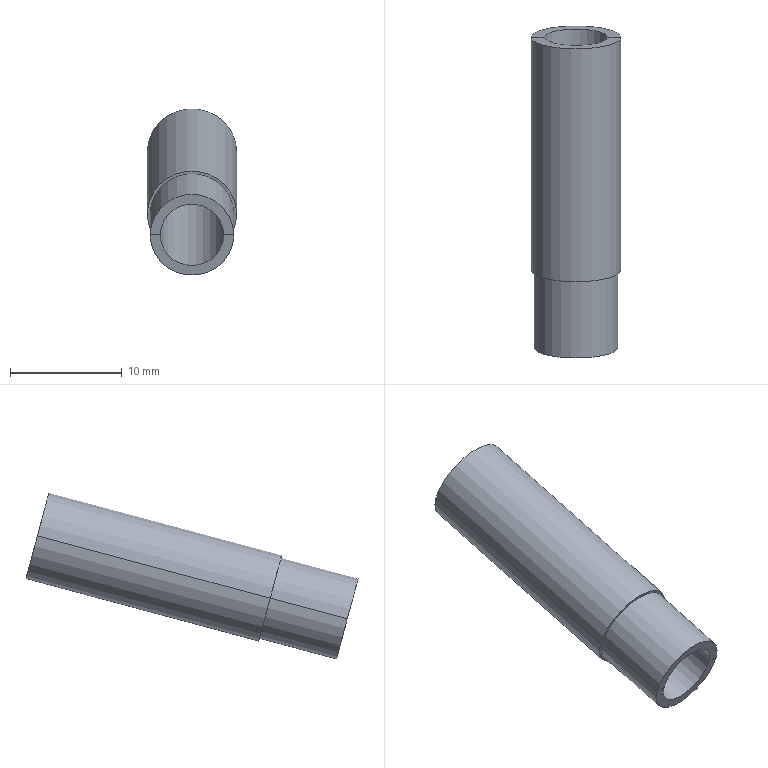Part | STEP file | BREP_2 | 1 solid | 12 faces | box 8 x 29.756 x 14.922 mm | volume 672.27 mm3 | cylinder 6 | plane 6 | commonest cylinder face diameters 5.681 x2 7.5 x2 8 x2
STEP:
#1=CARTESIAN_POINT('',(0.,0.,0.));
#2=DIRECTION('',(0.,0.,1.));
#3=DIRECTION('',(1.,0.,0.));
#4=AXIS2_PLACEMENT_3D('',#1,#2,#3);
#5=CARTESIAN_POINT('',(2.841,186.663,50.016));
#6=VERTEX_POINT('',#5);
#7=CARTESIAN_POINT('',(-2.841,186.663,50.016));
#8=VERTEX_POINT('',#7);
#9=CARTESIAN_POINT('',(0.,186.663,50.016));
#10=DIRECTION('',(0.,0.9659,0.2588));
#11=DIRECTION('',(1.,0.,0.));
#12=AXIS2_PLACEMENT_3D('',#9,#10,#11);
#13=CIRCLE('',#12,2.841);
#14=CARTESIAN_POINT('',(0.,200.538,53.734));
#15=DIRECTION('',(0.,0.9659,0.2588));
#16=DIRECTION('',(1.,0.,0.));
#17=AXIS2_PLACEMENT_3D('',#14,#15,#16);
#18=CYLINDRICAL_SURFACE('',#17,2.841);
#19=CARTESIAN_POINT('',(0.,-14.365));
#20=DIRECTION('',(1.,0.));
#21=VECTOR('',#20,1.);
#22=LINE('',#19,#21);
#23=(GEOMETRIC_REPRESENTATION_CONTEXT(2)PARAMETRIC_REPRESENTATION_CONTEXT()REPRESENTATION_CONTEXT('',''));
#24=DEFINITIONAL_REPRESENTATION('',(#22),#23);
#25=PCURVE('',#18,#24);
#26=CARTESIAN_POINT('',(0.,187.516,46.833));
#27=DIRECTION('',(0.,0.9659,0.2588));
#28=DIRECTION('',(0.,-0.2588,0.9659));
#29=AXIS2_PLACEMENT_3D('',#26,#27,#28);
#30=PLANE('',#29);
#31=CARTESIAN_POINT('',(3.295,0.));
#32=DIRECTION('',(0.,1.));
#33=AXIS2_PLACEMENT_2D('',#31,#32);
#34=CIRCLE('',#33,2.841);
#35=(GEOMETRIC_REPRESENTATION_CONTEXT(2)PARAMETRIC_REPRESENTATION_CONTEXT()REPRESENTATION_CONTEXT('',''));
#36=DEFINITIONAL_REPRESENTATION('',(#34),#35);
#37=PCURVE('',#30,#36);
#38=SURFACE_CURVE('',#13,(#25,#37),.PCURVE_S1.);
#39=EDGE_CURVE('',#6,#8,#38,.T.);
#40=ORIENTED_EDGE('',*,*,#39,.T.);
#41=CARTESIAN_POINT('',(-2.841,214.414,57.452));
#42=VERTEX_POINT('',#41);
#43=CARTESIAN_POINT('',(-2.841,214.414,57.452));
#44=DIRECTION('',(0.,-0.9659,-0.2588));
#45=VECTOR('',#44,1.);
#46=LINE('',#43,#45);
#47=CARTESIAN_POINT('',(3.142,14.365));
#48=DIRECTION('',(0.,-1.));
#49=VECTOR('',#48,1.);
#50=LINE('',#47,#49);
#51=(GEOMETRIC_REPRESENTATION_CONTEXT(2)PARAMETRIC_REPRESENTATION_CONTEXT()REPRESENTATION_CONTEXT('',''));
#52=DEFINITIONAL_REPRESENTATION('',(#50),#51);
#53=PCURVE('',#18,#52);
#54=CARTESIAN_POINT('',(0.,200.538,53.734));
#55=DIRECTION('',(0.,0.9659,0.2588));
#56=DIRECTION('',(-1.,0.,0.));
#57=AXIS2_PLACEMENT_3D('',#54,#55,#56);
#58=CYLINDRICAL_SURFACE('',#57,2.841);
#59=CARTESIAN_POINT('',(0.,14.365));
#60=DIRECTION('',(0.,-1.));
#61=VECTOR('',#60,1.);
#62=LINE('',#59,#61);
#63=(GEOMETRIC_REPRESENTATION_CONTEXT(2)PARAMETRIC_REPRESENTATION_CONTEXT()REPRESENTATION_CONTEXT('',''));
#64=DEFINITIONAL_REPRESENTATION('',(#62),#63);
#65=PCURVE('',#58,#64);
#66=SURFACE_CURVE('',#46,(#53,#65),.PCURVE_S1.);
#67=EDGE_CURVE('',#42,#8,#66,.T.);
#68=ORIENTED_EDGE('',*,*,#67,.F.);
#69=CARTESIAN_POINT('',(2.841,214.414,57.452));
#70=VERTEX_POINT('',#69);
#71=CARTESIAN_POINT('',(0.,214.414,57.452));
#72=DIRECTION('',(0.,-0.9659,-0.2588));
#73=DIRECTION('',(-1.,0.,0.));
#74=AXIS2_PLACEMENT_3D('',#71,#72,#73);
#75=CIRCLE('',#74,2.841);
#76=CARTESIAN_POINT('',(3.142,14.365));
#77=DIRECTION('',(-1.,0.));
#78=VECTOR('',#77,1.);
#79=LINE('',#76,#78);
#80=(GEOMETRIC_REPRESENTATION_CONTEXT(2)PARAMETRIC_REPRESENTATION_CONTEXT()REPRESENTATION_CONTEXT('',''));
#81=DEFINITIONAL_REPRESENTATION('',(#79),#80);
#82=PCURVE('',#18,#81);
#83=CARTESIAN_POINT('',(0.,215.299,54.148));
#84=DIRECTION('',(0.,0.9659,0.2588));
#85=DIRECTION('',(0.,0.2588,-0.9659));
#86=AXIS2_PLACEMENT_3D('',#83,#84,#85);
#87=PLANE('',#86);
#88=CARTESIAN_POINT('',(-3.42,2.841));
#89=CARTESIAN_POINT('',(1.5,2.841));
#90=CARTESIAN_POINT('',(-0.9602,-1.42));
#91=CARTESIAN_POINT('',(-3.42,-5.681));
#92=CARTESIAN_POINT('',(-5.88,-1.42));
#93=CARTESIAN_POINT('',(-8.341,2.841));
#94=CARTESIAN_POINT('',(-3.42,2.841));
#95=(BOUNDED_CURVE()B_SPLINE_CURVE(2,(#88,#89,#90,#91,#92,#93,#94),.UNSPECIFIED.,.T.,.F.)B_SPLINE_CURVE_WITH_KNOTS((1,2,2,2,2,1),(-2.094,0.,2.094,4.189,6.283,8.378),.UNSPECIFIED.)CURVE()GEOMETRIC_REPRESENTATION_ITEM()RATIONAL_B_SPLINE_CURVE((1.,0.5,1.,0.5,1.,0.5,1.))REPRESENTATION_ITEM(''));
#96=(GEOMETRIC_REPRESENTATION_CONTEXT(2)PARAMETRIC_REPRESENTATION_CONTEXT()REPRESENTATION_CONTEXT('',''));
#97=DEFINITIONAL_REPRESENTATION('',(#95),#96);
#98=PCURVE('',#87,#97);
#99=SURFACE_CURVE('',#75,(#82,#98),.PCURVE_S1.);
#100=EDGE_CURVE('',#42,#70,#99,.T.);
#101=ORIENTED_EDGE('',*,*,#100,.T.);
#102=CARTESIAN_POINT('',(2.841,214.414,57.452));
#103=DIRECTION('',(0.,-0.9659,-0.2588));
#104=VECTOR('',#103,1.);
#105=LINE('',#102,#104);
#106=CARTESIAN_POINT('',(0.,14.365));
#107=DIRECTION('',(0.,-1.));
#108=VECTOR('',#107,1.);
#109=LINE('',#106,#108);
#110=(GEOMETRIC_REPRESENTATION_CONTEXT(2)PARAMETRIC_REPRESENTATION_CONTEXT()REPRESENTATION_CONTEXT('',''));
#111=DEFINITIONAL_REPRESENTATION('',(#109),#110);
#112=PCURVE('',#18,#111);
#113=CARTESIAN_POINT('',(3.142,14.365));
#114=DIRECTION('',(0.,-1.));
#115=VECTOR('',#114,1.);
#116=LINE('',#113,#115);
#117=(GEOMETRIC_REPRESENTATION_CONTEXT(2)PARAMETRIC_REPRESENTATION_CONTEXT()REPRESENTATION_CONTEXT('',''));
#118=DEFINITIONAL_REPRESENTATION('',(#116),#117);
#119=PCURVE('',#58,#118);
#120=SURFACE_CURVE('',#105,(#112,#119),.PCURVE_S1.);
#121=EDGE_CURVE('',#70,#6,#120,.T.);
#122=ORIENTED_EDGE('',*,*,#121,.T.);
#123=EDGE_LOOP('',(#40,#68,#101,#122));
#124=FACE_BOUND('',#123,.F.);
#125=ADVANCED_FACE('',(#124),#18,.F.);
#126=CARTESIAN_POINT('',(-3.75,186.663,50.016));
#127=VERTEX_POINT('',#126);
#128=CARTESIAN_POINT('',(3.75,186.663,50.016));
#129=VERTEX_POINT('',#128);
#130=CARTESIAN_POINT('',(0.,186.663,50.016));
#131=DIRECTION('',(0.,-0.9659,-0.2588));
#132=DIRECTION('',(-1.,0.,0.));
#133=AXIS2_PLACEMENT_3D('',#130,#131,#132);
#134=CIRCLE('',#133,3.75);
#135=CARTESIAN_POINT('',(3.295,-3.75));
#136=CARTESIAN_POINT('',(-3.2,-3.75));
#137=CARTESIAN_POINT('',(0.04775,1.875));
#138=CARTESIAN_POINT('',(3.295,7.5));
#139=CARTESIAN_POINT('',(6.543,1.875));
#140=CARTESIAN_POINT('',(9.791,-3.75));
#141=CARTESIAN_POINT('',(3.295,-3.75));
#142=(BOUNDED_CURVE()B_SPLINE_CURVE(2,(#135,#136,#137,#138,#139,#140,#141),.UNSPECIFIED.,.T.,.F.)B_SPLINE_CURVE_WITH_KNOTS((1,2,2,2,2,1),(-2.094,0.,2.094,4.189,6.283,8.378),.UNSPECIFIED.)CURVE()GEOMETRIC_REPRESENTATION_ITEM()RATIONAL_B_SPLINE_CURVE((1.,0.5,1.,0.5,1.,0.5,1.))REPRESENTATION_ITEM(''));
#143=(GEOMETRIC_REPRESENTATION_CONTEXT(2)PARAMETRIC_REPRESENTATION_CONTEXT()REPRESENTATION_CONTEXT('',''));
#144=DEFINITIONAL_REPRESENTATION('',(#142),#143);
#145=PCURVE('',#30,#144);
#146=CARTESIAN_POINT('',(0.,190.115,50.941));
#147=DIRECTION('',(0.,-0.9659,-0.2588));
#148=DIRECTION('',(1.,0.,0.));
#149=AXIS2_PLACEMENT_3D('',#146,#147,#148);
#150=CYLINDRICAL_SURFACE('',#149,3.75);
#151=CARTESIAN_POINT('',(3.142,3.573));
#152=DIRECTION('',(1.,0.));
#153=VECTOR('',#152,1.);
#154=LINE('',#151,#153);
#155=(GEOMETRIC_REPRESENTATION_CONTEXT(2)PARAMETRIC_REPRESENTATION_CONTEXT()REPRESENTATION_CONTEXT('',''));
#156=DEFINITIONAL_REPRESENTATION('',(#154),#155);
#157=PCURVE('',#150,#156);
#158=SURFACE_CURVE('',#134,(#145,#157),.PCURVE_S1.);
#159=EDGE_CURVE('',#127,#129,#158,.T.);
#160=ORIENTED_EDGE('',*,*,#159,.F.);
#161=CARTESIAN_POINT('',(-2.841,186.663,50.016));
#162=DIRECTION('',(-1.,0.,0.));
#163=VECTOR('',#162,1.);
#164=LINE('',#161,#163);
#165=CARTESIAN_POINT('',(3.295,-2.841));
#166=DIRECTION('',(0.,-1.));
#167=VECTOR('',#166,1.);
#168=LINE('',#165,#167);
#169=(GEOMETRIC_REPRESENTATION_CONTEXT(2)PARAMETRIC_REPRESENTATION_CONTEXT()REPRESENTATION_CONTEXT('',''));
#170=DEFINITIONAL_REPRESENTATION('',(#168),#169);
#171=PCURVE('',#30,#170);
#172=CARTESIAN_POINT('',(0.,185.81,53.199));
#173=DIRECTION('',(0.,0.9659,0.2588));
#174=DIRECTION('',(0.,0.2588,-0.9659));
#175=AXIS2_PLACEMENT_3D('',#172,#173,#174);
#176=PLANE('',#175);
#177=CARTESIAN_POINT('',(3.295,2.841));
#178=DIRECTION('',(0.,1.));
#179=VECTOR('',#178,1.);
#180=LINE('',#177,#179);
#181=(GEOMETRIC_REPRESENTATION_CONTEXT(2)PARAMETRIC_REPRESENTATION_CONTEXT()REPRESENTATION_CONTEXT('',''));
#182=DEFINITIONAL_REPRESENTATION('',(#180),#181);
#183=PCURVE('',#176,#182);
#184=SURFACE_CURVE('',#164,(#171,#183),.PCURVE_S1.);
#185=EDGE_CURVE('',#8,#127,#184,.T.);
#186=ORIENTED_EDGE('',*,*,#185,.F.);
#187=ORIENTED_EDGE('',*,*,#39,.F.);
#188=CARTESIAN_POINT('',(2.841,186.663,50.016));
#189=DIRECTION('',(1.,0.,0.));
#190=VECTOR('',#189,1.);
#191=LINE('',#188,#190);
#192=CARTESIAN_POINT('',(3.295,2.841));
#193=DIRECTION('',(0.,1.));
#194=VECTOR('',#193,1.);
#195=LINE('',#192,#194);
#196=(GEOMETRIC_REPRESENTATION_CONTEXT(2)PARAMETRIC_REPRESENTATION_CONTEXT()REPRESENTATION_CONTEXT('',''));
#197=DEFINITIONAL_REPRESENTATION('',(#195),#196);
#198=PCURVE('',#30,#197);
#199=CARTESIAN_POINT('',(3.295,-2.841));
#200=DIRECTION('',(0.,-1.));
#201=VECTOR('',#200,1.);
#202=LINE('',#199,#201);
#203=(GEOMETRIC_REPRESENTATION_CONTEXT(2)PARAMETRIC_REPRESENTATION_CONTEXT()REPRESENTATION_CONTEXT('',''));
#204=DEFINITIONAL_REPRESENTATION('',(#202),#203);
#205=PCURVE('',#176,#204);
#206=SURFACE_CURVE('',#191,(#198,#205),.PCURVE_S1.);
#207=EDGE_CURVE('',#6,#129,#206,.T.);
#208=ORIENTED_EDGE('',*,*,#207,.T.);
#209=EDGE_LOOP('',(#160,#186,#187,#208));
#210=FACE_BOUND('',#209,.F.);
#211=ADVANCED_FACE('',(#210),#30,.F.);
#212=CARTESIAN_POINT('',(3.75,193.567,51.866));
#213=VERTEX_POINT('',#212);
#214=CARTESIAN_POINT('',(3.75,186.663,50.016));
#215=DIRECTION('',(0.,0.9659,0.2588));
#216=VECTOR('',#215,1.);
#217=LINE('',#214,#216);
#218=CARTESIAN_POINT('',(6.283,3.573));
#219=DIRECTION('',(0.,-1.));
#220=VECTOR('',#219,1.);
#221=LINE('',#218,#220);
#222=(GEOMETRIC_REPRESENTATION_CONTEXT(2)PARAMETRIC_REPRESENTATION_CONTEXT()REPRESENTATION_CONTEXT('',''));
#223=DEFINITIONAL_REPRESENTATION('',(#221),#222);
#224=PCURVE('',#150,#223);
#225=CARTESIAN_POINT('',(0.,190.115,50.941));
#226=DIRECTION('',(0.,-0.9659,-0.2588));
#227=DIRECTION('',(-1.,0.,0.));
#228=AXIS2_PLACEMENT_3D('',#225,#226,#227);
#229=CYLINDRICAL_SURFACE('',#228,3.75);
#230=CARTESIAN_POINT('',(3.142,3.573));
#231=DIRECTION('',(0.,-1.));
#232=VECTOR('',#231,1.);
#233=LINE('',#230,#232);
#234=(GEOMETRIC_REPRESENTATION_CONTEXT(2)PARAMETRIC_REPRESENTATION_CONTEXT()REPRESENTATION_CONTEXT('',''));
#235=DEFINITIONAL_REPRESENTATION('',(#233),#234);
#236=PCURVE('',#229,#235);
#237=SURFACE_CURVE('',#217,(#224,#236),.PCURVE_S1.);
#238=EDGE_CURVE('',#129,#213,#237,.T.);
#239=ORIENTED_EDGE('',*,*,#238,.F.);
#240=ORIENTED_EDGE('',*,*,#159,.F.);
#241=CARTESIAN_POINT('',(-3.75,193.567,51.866));
#242=VERTEX_POINT('',#241);
#243=CARTESIAN_POINT('',(-3.75,186.663,50.016));
#244=DIRECTION('',(0.,0.9659,0.2588));
#245=VECTOR('',#244,1.);
#246=LINE('',#243,#245);
#247=CARTESIAN_POINT('',(3.142,3.573));
#248=DIRECTION('',(0.,-1.));
#249=VECTOR('',#248,1.);
#250=LINE('',#247,#249);
#251=(GEOMETRIC_REPRESENTATION_CONTEXT(2)PARAMETRIC_REPRESENTATION_CONTEXT()REPRESENTATION_CONTEXT('',''));
#252=DEFINITIONAL_REPRESENTATION('',(#250),#251);
#253=PCURVE('',#150,#252);
#254=CARTESIAN_POINT('',(6.283,3.573));
#255=DIRECTION('',(0.,-1.));
#256=VECTOR('',#255,1.);
#257=LINE('',#254,#256);
#258=(GEOMETRIC_REPRESENTATION_CONTEXT(2)PARAMETRIC_REPRESENTATION_CONTEXT()REPRESENTATION_CONTEXT('',''));
#259=DEFINITIONAL_REPRESENTATION('',(#257),#258);
#260=PCURVE('',#229,#259);
#261=SURFACE_CURVE('',#246,(#253,#260),.PCURVE_S1.);
#262=EDGE_CURVE('',#127,#242,#261,.T.);
#263=ORIENTED_EDGE('',*,*,#262,.T.);
#264=CARTESIAN_POINT('',(0.,193.567,51.866));
#265=DIRECTION('',(0.,0.9659,0.2588));
#266=DIRECTION('',(1.,0.,0.));
#267=AXIS2_PLACEMENT_3D('',#264,#265,#266);
#268=CIRCLE('',#267,3.75);
#269=CARTESIAN_POINT('',(6.283,-3.573));
#270=DIRECTION('',(-1.,0.));
#271=VECTOR('',#270,1.);
#272=LINE('',#269,#271);
#273=(GEOMETRIC_REPRESENTATION_CONTEXT(2)PARAMETRIC_REPRESENTATION_CONTEXT()REPRESENTATION_CONTEXT('',''));
#274=DEFINITIONAL_REPRESENTATION('',(#272),#273);
#275=PCURVE('',#150,#274);
#276=CARTESIAN_POINT('',(0.,194.57,48.123));
#277=DIRECTION('',(0.,0.9659,0.2588));
#278=DIRECTION('',(0.,-0.2588,0.9659));
#279=AXIS2_PLACEMENT_3D('',#276,#277,#278);
#280=PLANE('',#279);
#281=CARTESIAN_POINT('',(3.875,0.));
#282=DIRECTION('',(0.,1.));
#283=AXIS2_PLACEMENT_2D('',#281,#282);
#284=CIRCLE('',#283,3.75);
#285=(GEOMETRIC_REPRESENTATION_CONTEXT(2)PARAMETRIC_REPRESENTATION_CONTEXT()REPRESENTATION_CONTEXT('',''));
#286=DEFINITIONAL_REPRESENTATION('',(#284),#285);
#287=PCURVE('',#280,#286);
#288=SURFACE_CURVE('',#268,(#275,#287),.PCURVE_S1.);
#289=EDGE_CURVE('',#213,#242,#288,.T.);
#290=ORIENTED_EDGE('',*,*,#289,.F.);
#291=EDGE_LOOP('',(#239,#240,#263,#290));
#292=FACE_BOUND('',#291,.T.);
#293=ADVANCED_FACE('',(#292),#150,.T.);
#294=CARTESIAN_POINT('',(-4.,193.567,51.866));
#295=VERTEX_POINT('',#294);
#296=CARTESIAN_POINT('',(4.,193.567,51.866));
#297=VERTEX_POINT('',#296);
#298=CARTESIAN_POINT('',(0.,193.567,51.866));
#299=DIRECTION('',(0.,-0.9659,-0.2588));
#300=DIRECTION('',(-1.,0.,0.));
#301=AXIS2_PLACEMENT_3D('',#298,#299,#300);
#302=CIRCLE('',#301,4.);
#303=CARTESIAN_POINT('',(3.875,-4.));
#304=CARTESIAN_POINT('',(-3.053,-4.));
#305=CARTESIAN_POINT('',(0.4109,2.));
#306=CARTESIAN_POINT('',(3.875,8.));
#307=CARTESIAN_POINT('',(7.339,2.));
#308=CARTESIAN_POINT('',(10.803,-4.));
#309=CARTESIAN_POINT('',(3.875,-4.));
#310=(BOUNDED_CURVE()B_SPLINE_CURVE(2,(#303,#304,#305,#306,#307,#308,#309),.UNSPECIFIED.,.T.,.F.)B_SPLINE_CURVE_WITH_KNOTS((1,2,2,2,2,1),(-2.094,0.,2.094,4.189,6.283,8.378),.UNSPECIFIED.)CURVE()GEOMETRIC_REPRESENTATION_ITEM()RATIONAL_B_SPLINE_CURVE((1.,0.5,1.,0.5,1.,0.5,1.))REPRESENTATION_ITEM(''));
#311=(GEOMETRIC_REPRESENTATION_CONTEXT(2)PARAMETRIC_REPRESENTATION_CONTEXT()REPRESENTATION_CONTEXT('',''));
#312=DEFINITIONAL_REPRESENTATION('',(#310),#311);
#313=PCURVE('',#280,#312);
#314=CARTESIAN_POINT('',(0.,203.99,54.659));
#315=DIRECTION('',(0.,-0.9659,-0.2588));
#316=DIRECTION('',(1.,0.,0.));
#317=AXIS2_PLACEMENT_3D('',#314,#315,#316);
#318=CYLINDRICAL_SURFACE('',#317,4.);
#319=CARTESIAN_POINT('',(3.142,10.791));
#320=DIRECTION('',(1.,0.));
#321=VECTOR('',#320,1.);
#322=LINE('',#319,#321);
#323=(GEOMETRIC_REPRESENTATION_CONTEXT(2)PARAMETRIC_REPRESENTATION_CONTEXT()REPRESENTATION_CONTEXT('',''));
#324=DEFINITIONAL_REPRESENTATION('',(#322),#323);
#325=PCURVE('',#318,#324);
#326=SURFACE_CURVE('',#302,(#313,#325),.PCURVE_S1.);
#327=EDGE_CURVE('',#295,#297,#326,.T.);
#328=ORIENTED_EDGE('',*,*,#327,.F.);
#329=CARTESIAN_POINT('',(-3.75,193.567,51.866));
#330=DIRECTION('',(-1.,0.,0.));
#331=VECTOR('',#330,1.);
#332=LINE('',#329,#331);
#333=CARTESIAN_POINT('',(3.875,-3.75));
#334=DIRECTION('',(0.,-1.));
#335=VECTOR('',#334,1.);
#336=LINE('',#333,#335);
#337=(GEOMETRIC_REPRESENTATION_CONTEXT(2)PARAMETRIC_REPRESENTATION_CONTEXT()REPRESENTATION_CONTEXT('',''));
#338=DEFINITIONAL_REPRESENTATION('',(#336),#337);
#339=PCURVE('',#280,#338);
#340=CARTESIAN_POINT('',(0.,192.564,55.609));
#341=DIRECTION('',(0.,0.9659,0.2588));
#342=DIRECTION('',(0.,0.2588,-0.9659));
#343=AXIS2_PLACEMENT_3D('',#340,#341,#342);
#344=PLANE('',#343);
#345=CARTESIAN_POINT('',(3.875,3.75));
#346=DIRECTION('',(0.,1.));
#347=VECTOR('',#346,1.);
#348=LINE('',#345,#347);
#349=(GEOMETRIC_REPRESENTATION_CONTEXT(2)PARAMETRIC_REPRESENTATION_CONTEXT()REPRESENTATION_CONTEXT('',''));
#350=DEFINITIONAL_REPRESENTATION('',(#348),#349);
#351=PCURVE('',#344,#350);
#352=SURFACE_CURVE('',#332,(#339,#351),.PCURVE_S1.);
#353=EDGE_CURVE('',#242,#295,#352,.T.);
#354=ORIENTED_EDGE('',*,*,#353,.F.);
#355=ORIENTED_EDGE('',*,*,#289,.F.);
#356=CARTESIAN_POINT('',(3.75,193.567,51.866));
#357=DIRECTION('',(1.,0.,0.));
#358=VECTOR('',#357,1.);
#359=LINE('',#356,#358);
#360=CARTESIAN_POINT('',(3.875,3.75));
#361=DIRECTION('',(0.,1.));
#362=VECTOR('',#361,1.);
#363=LINE('',#360,#362);
#364=(GEOMETRIC_REPRESENTATION_CONTEXT(2)PARAMETRIC_REPRESENTATION_CONTEXT()REPRESENTATION_CONTEXT('',''));
#365=DEFINITIONAL_REPRESENTATION('',(#363),#364);
#366=PCURVE('',#280,#365);
#367=CARTESIAN_POINT('',(3.875,-3.75));
#368=DIRECTION('',(0.,-1.));
#369=VECTOR('',#368,1.);
#370=LINE('',#367,#369);
#371=(GEOMETRIC_REPRESENTATION_CONTEXT(2)PARAMETRIC_REPRESENTATION_CONTEXT()REPRESENTATION_CONTEXT('',''));
#372=DEFINITIONAL_REPRESENTATION('',(#370),#371);
#373=PCURVE('',#344,#372);
#374=SURFACE_CURVE('',#359,(#366,#373),.PCURVE_S1.);
#375=EDGE_CURVE('',#213,#297,#374,.T.);
#376=ORIENTED_EDGE('',*,*,#375,.T.);
#377=EDGE_LOOP('',(#328,#354,#355,#376));
#378=FACE_BOUND('',#377,.F.);
#379=ADVANCED_FACE('',(#378),#280,.F.);
#380=CARTESIAN_POINT('',(4.,214.414,57.452));
#381=VERTEX_POINT('',#380);
#382=CARTESIAN_POINT('',(4.,193.567,51.866));
#383=DIRECTION('',(0.,0.9659,0.2588));
#384=VECTOR('',#383,1.);
#385=LINE('',#382,#384);
#386=CARTESIAN_POINT('',(6.283,10.791));
#387=DIRECTION('',(0.,-1.));
#388=VECTOR('',#387,1.);
#389=LINE('',#386,#388);
#390=(GEOMETRIC_REPRESENTATION_CONTEXT(2)PARAMETRIC_REPRESENTATION_CONTEXT()REPRESENTATION_CONTEXT('',''));
#391=DEFINITIONAL_REPRESENTATION('',(#389),#390);
#392=PCURVE('',#318,#391);
#393=CARTESIAN_POINT('',(0.,203.99,54.659));
#394=DIRECTION('',(0.,-0.9659,-0.2588));
#395=DIRECTION('',(-1.,0.,0.));
#396=AXIS2_PLACEMENT_3D('',#393,#394,#395);
#397=CYLINDRICAL_SURFACE('',#396,4.);
#398=CARTESIAN_POINT('',(3.142,10.791));
#399=DIRECTION('',(0.,-1.));
#400=VECTOR('',#399,1.);
#401=LINE('',#398,#400);
#402=(GEOMETRIC_REPRESENTATION_CONTEXT(2)PARAMETRIC_REPRESENTATION_CONTEXT()REPRESENTATION_CONTEXT('',''));
#403=DEFINITIONAL_REPRESENTATION('',(#401),#402);
#404=PCURVE('',#397,#403);
#405=SURFACE_CURVE('',#385,(#392,#404),.PCURVE_S1.);
#406=EDGE_CURVE('',#297,#381,#405,.T.);
#407=ORIENTED_EDGE('',*,*,#406,.F.);
#408=ORIENTED_EDGE('',*,*,#327,.F.);
#409=CARTESIAN_POINT('',(-4.,214.414,57.452));
#410=VERTEX_POINT('',#409);
#411=CARTESIAN_POINT('',(-4.,193.567,51.866));
#412=DIRECTION('',(0.,0.9659,0.2588));
#413=VECTOR('',#412,1.);
#414=LINE('',#411,#413);
#415=CARTESIAN_POINT('',(3.142,10.791));
#416=DIRECTION('',(0.,-1.));
#417=VECTOR('',#416,1.);
#418=LINE('',#415,#417);
#419=(GEOMETRIC_REPRESENTATION_CONTEXT(2)PARAMETRIC_REPRESENTATION_CONTEXT()REPRESENTATION_CONTEXT('',''));
#420=DEFINITIONAL_REPRESENTATION('',(#418),#419);
#421=PCURVE('',#318,#420);
#422=CARTESIAN_POINT('',(6.283,10.791));
#423=DIRECTION('',(0.,-1.));
#424=VECTOR('',#423,1.);
#425=LINE('',#422,#424);
#426=(GEOMETRIC_REPRESENTATION_CONTEXT(2)PARAMETRIC_REPRESENTATION_CONTEXT()REPRESENTATION_CONTEXT('',''));
#427=DEFINITIONAL_REPRESENTATION('',(#425),#426);
#428=PCURVE('',#397,#427);
#429=SURFACE_CURVE('',#414,(#421,#428),.PCURVE_S1.);
#430=EDGE_CURVE('',#295,#410,#429,.T.);
#431=ORIENTED_EDGE('',*,*,#430,.T.);
#432=CARTESIAN_POINT('',(0.,214.414,57.452));
#433=DIRECTION('',(0.,0.9659,0.2588));
#434=DIRECTION('',(1.,0.,0.));
#435=AXIS2_PLACEMENT_3D('',#432,#433,#434);
#436=CIRCLE('',#435,4.);
#437=CARTESIAN_POINT('',(6.283,-10.791));
#438=DIRECTION('',(-1.,0.));
#439=VECTOR('',#438,1.);
#440=LINE('',#437,#439);
#441=(GEOMETRIC_REPRESENTATION_CONTEXT(2)PARAMETRIC_REPRESENTATION_CONTEXT()REPRESENTATION_CONTEXT('',''));
#442=DEFINITIONAL_REPRESENTATION('',(#440),#441);
#443=PCURVE('',#318,#442);
#444=CARTESIAN_POINT('',(-3.42,0.));
#445=DIRECTION('',(0.,-1.));
#446=AXIS2_PLACEMENT_2D('',#444,#445);
#447=CIRCLE('',#446,4.);
#448=(GEOMETRIC_REPRESENTATION_CONTEXT(2)PARAMETRIC_REPRESENTATION_CONTEXT()REPRESENTATION_CONTEXT('',''));
#449=DEFINITIONAL_REPRESENTATION('',(#447),#448);
#450=PCURVE('',#87,#449);
#451=SURFACE_CURVE('',#436,(#443,#450),.PCURVE_S1.);
#452=EDGE_CURVE('',#381,#410,#451,.T.);
#453=ORIENTED_EDGE('',*,*,#452,.F.);
#454=EDGE_LOOP('',(#407,#408,#431,#453));
#455=FACE_BOUND('',#454,.T.);
#456=ADVANCED_FACE('',(#455),#318,.T.);
#457=ORIENTED_EDGE('',*,*,#100,.F.);
#458=CARTESIAN_POINT('',(-4.,214.414,57.452));
#459=DIRECTION('',(1.,0.,0.));
#460=VECTOR('',#459,1.);
#461=LINE('',#458,#460);
#462=CARTESIAN_POINT('',(-3.42,4.));
#463=DIRECTION('',(0.,-1.));
#464=VECTOR('',#463,1.);
#465=LINE('',#462,#464);
#466=(GEOMETRIC_REPRESENTATION_CONTEXT(2)PARAMETRIC_REPRESENTATION_CONTEXT()REPRESENTATION_CONTEXT('',''));
#467=DEFINITIONAL_REPRESENTATION('',(#465),#466);
#468=PCURVE('',#87,#467);
#469=CARTESIAN_POINT('',(0.,213.528,60.756));
#470=DIRECTION('',(0.,0.9659,0.2588));
#471=DIRECTION('',(0.,-0.2588,0.9659));
#472=AXIS2_PLACEMENT_3D('',#469,#470,#471);
#473=PLANE('',#472);
#474=CARTESIAN_POINT('',(-3.42,-4.));
#475=DIRECTION('',(0.,1.));
#476=VECTOR('',#475,1.);
#477=LINE('',#474,#476);
#478=(GEOMETRIC_REPRESENTATION_CONTEXT(2)PARAMETRIC_REPRESENTATION_CONTEXT()REPRESENTATION_CONTEXT('',''));
#479=DEFINITIONAL_REPRESENTATION('',(#477),#478);
#480=PCURVE('',#473,#479);
#481=SURFACE_CURVE('',#461,(#468,#480),.PCURVE_S1.);
#482=EDGE_CURVE('',#410,#42,#481,.T.);
#483=ORIENTED_EDGE('',*,*,#482,.F.);
#484=ORIENTED_EDGE('',*,*,#452,.F.);
#485=CARTESIAN_POINT('',(4.,214.414,57.452));
#486=DIRECTION('',(-1.,0.,0.));
#487=VECTOR('',#486,1.);
#488=LINE('',#485,#487);
#489=CARTESIAN_POINT('',(-3.42,-4.));
#490=DIRECTION('',(0.,1.));
#491=VECTOR('',#490,1.);
#492=LINE('',#489,#491);
#493=(GEOMETRIC_REPRESENTATION_CONTEXT(2)PARAMETRIC_REPRESENTATION_CONTEXT()REPRESENTATION_CONTEXT('',''));
#494=DEFINITIONAL_REPRESENTATION('',(#492),#493);
#495=PCURVE('',#87,#494);
#496=CARTESIAN_POINT('',(-3.42,4.));
#497=DIRECTION('',(0.,-1.));
#498=VECTOR('',#497,1.);
#499=LINE('',#496,#498);
#500=(GEOMETRIC_REPRESENTATION_CONTEXT(2)PARAMETRIC_REPRESENTATION_CONTEXT()REPRESENTATION_CONTEXT('',''));
#501=DEFINITIONAL_REPRESENTATION('',(#499),#500);
#502=PCURVE('',#473,#501);
#503=SURFACE_CURVE('',#488,(#495,#502),.PCURVE_S1.);
#504=EDGE_CURVE('',#381,#70,#503,.T.);
#505=ORIENTED_EDGE('',*,*,#504,.T.);
#506=EDGE_LOOP('',(#457,#483,#484,#505));
#507=FACE_BOUND('',#506,.F.);
#508=ADVANCED_FACE('',(#507),#87,.T.);
#509=ORIENTED_EDGE('',*,*,#482,.T.);
#510=CARTESIAN_POINT('',(0.,214.414,57.452));
#511=DIRECTION('',(0.,-0.9659,-0.2588));
#512=DIRECTION('',(1.,0.,0.));
#513=AXIS2_PLACEMENT_3D('',#510,#511,#512);
#514=CIRCLE('',#513,2.841);
#515=CARTESIAN_POINT('',(-3.42,2.841));
#516=CARTESIAN_POINT('',(1.5,2.841));
#517=CARTESIAN_POINT('',(-0.9602,-1.42));
#518=CARTESIAN_POINT('',(-3.42,-5.681));
#519=CARTESIAN_POINT('',(-5.88,-1.42));
#520=CARTESIAN_POINT('',(-8.341,2.841));
#521=CARTESIAN_POINT('',(-3.42,2.841));
#522=(BOUNDED_CURVE()B_SPLINE_CURVE(2,(#515,#516,#517,#518,#519,#520,#521),.UNSPECIFIED.,.T.,.F.)B_SPLINE_CURVE_WITH_KNOTS((1,2,2,2,2,1),(-2.094,0.,2.094,4.189,6.283,8.378),.UNSPECIFIED.)CURVE()GEOMETRIC_REPRESENTATION_ITEM()RATIONAL_B_SPLINE_CURVE((1.,0.5,1.,0.5,1.,0.5,1.))REPRESENTATION_ITEM(''));
#523=(GEOMETRIC_REPRESENTATION_CONTEXT(2)PARAMETRIC_REPRESENTATION_CONTEXT()REPRESENTATION_CONTEXT('',''));
#524=DEFINITIONAL_REPRESENTATION('',(#522),#523);
#525=PCURVE('',#473,#524);
#526=CARTESIAN_POINT('',(3.142,14.365));
#527=DIRECTION('',(-1.,0.));
#528=VECTOR('',#527,1.);
#529=LINE('',#526,#528);
#530=(GEOMETRIC_REPRESENTATION_CONTEXT(2)PARAMETRIC_REPRESENTATION_CONTEXT()REPRESENTATION_CONTEXT('',''));
#531=DEFINITIONAL_REPRESENTATION('',(#529),#530);
#532=PCURVE('',#58,#531);
#533=SURFACE_CURVE('',#514,(#525,#532),.PCURVE_S1.);
#534=EDGE_CURVE('',#70,#42,#533,.T.);
#535=ORIENTED_EDGE('',*,*,#534,.F.);
#536=ORIENTED_EDGE('',*,*,#504,.F.);
#537=CARTESIAN_POINT('',(0.,214.414,57.452));
#538=DIRECTION('',(0.,0.9659,0.2588));
#539=DIRECTION('',(-1.,0.,0.));
#540=AXIS2_PLACEMENT_3D('',#537,#538,#539);
#541=CIRCLE('',#540,4.);
#542=CARTESIAN_POINT('',(-3.42,0.));
#543=DIRECTION('',(0.,-1.));
#544=AXIS2_PLACEMENT_2D('',#542,#543);
#545=CIRCLE('',#544,4.);
#546=(GEOMETRIC_REPRESENTATION_CONTEXT(2)PARAMETRIC_REPRESENTATION_CONTEXT()REPRESENTATION_CONTEXT('',''));
#547=DEFINITIONAL_REPRESENTATION('',(#545),#546);
#548=PCURVE('',#473,#547);
#549=CARTESIAN_POINT('',(6.283,-10.791));
#550=DIRECTION('',(-1.,0.));
#551=VECTOR('',#550,1.);
#552=LINE('',#549,#551);
#553=(GEOMETRIC_REPRESENTATION_CONTEXT(2)PARAMETRIC_REPRESENTATION_CONTEXT()REPRESENTATION_CONTEXT('',''));
#554=DEFINITIONAL_REPRESENTATION('',(#552),#553);
#555=PCURVE('',#397,#554);
#556=SURFACE_CURVE('',#541,(#548,#555),.PCURVE_S1.);
#557=EDGE_CURVE('',#410,#381,#556,.T.);
#558=ORIENTED_EDGE('',*,*,#557,.F.);
#559=EDGE_LOOP('',(#509,#535,#536,#558));
#560=FACE_BOUND('',#559,.F.);
#561=ADVANCED_FACE('',(#560),#473,.T.);
#562=ORIENTED_EDGE('',*,*,#67,.T.);
#563=CARTESIAN_POINT('',(0.,186.663,50.016));
#564=DIRECTION('',(0.,0.9659,0.2588));
#565=DIRECTION('',(-1.,0.,0.));
#566=AXIS2_PLACEMENT_3D('',#563,#564,#565);
#567=CIRCLE('',#566,2.841);
#568=CARTESIAN_POINT('',(0.,-14.365));
#569=DIRECTION('',(1.,0.));
#570=VECTOR('',#569,1.);
#571=LINE('',#568,#570);
#572=(GEOMETRIC_REPRESENTATION_CONTEXT(2)PARAMETRIC_REPRESENTATION_CONTEXT()REPRESENTATION_CONTEXT('',''));
#573=DEFINITIONAL_REPRESENTATION('',(#571),#572);
#574=PCURVE('',#58,#573);
#575=CARTESIAN_POINT('',(3.295,0.));
#576=DIRECTION('',(0.,1.));
#577=AXIS2_PLACEMENT_2D('',#575,#576);
#578=CIRCLE('',#577,2.841);
#579=(GEOMETRIC_REPRESENTATION_CONTEXT(2)PARAMETRIC_REPRESENTATION_CONTEXT()REPRESENTATION_CONTEXT('',''));
#580=DEFINITIONAL_REPRESENTATION('',(#578),#579);
#581=PCURVE('',#176,#580);
#582=SURFACE_CURVE('',#567,(#574,#581),.PCURVE_S1.);
#583=EDGE_CURVE('',#8,#6,#582,.T.);
#584=ORIENTED_EDGE('',*,*,#583,.T.);
#585=ORIENTED_EDGE('',*,*,#121,.F.);
#586=ORIENTED_EDGE('',*,*,#534,.T.);
#587=EDGE_LOOP('',(#562,#584,#585,#586));
#588=FACE_BOUND('',#587,.F.);
#589=ADVANCED_FACE('',(#588),#58,.F.);
#590=ORIENTED_EDGE('',*,*,#185,.T.);
#591=CARTESIAN_POINT('',(0.,186.663,50.016));
#592=DIRECTION('',(0.,-0.9659,-0.2588));
#593=DIRECTION('',(1.,0.,0.));
#594=AXIS2_PLACEMENT_3D('',#591,#592,#593);
#595=CIRCLE('',#594,3.75);
#596=CARTESIAN_POINT('',(3.295,-3.75));
#597=CARTESIAN_POINT('',(-3.2,-3.75));
#598=CARTESIAN_POINT('',(0.04775,1.875));
#599=CARTESIAN_POINT('',(3.295,7.5));
#600=CARTESIAN_POINT('',(6.543,1.875));
#601=CARTESIAN_POINT('',(9.791,-3.75));
#602=CARTESIAN_POINT('',(3.295,-3.75));
#603=(BOUNDED_CURVE()B_SPLINE_CURVE(2,(#596,#597,#598,#599,#600,#601,#602),.UNSPECIFIED.,.T.,.F.)B_SPLINE_CURVE_WITH_KNOTS((1,2,2,2,2,1),(-2.094,0.,2.094,4.189,6.283,8.378),.UNSPECIFIED.)CURVE()GEOMETRIC_REPRESENTATION_ITEM()RATIONAL_B_SPLINE_CURVE((1.,0.5,1.,0.5,1.,0.5,1.))REPRESENTATION_ITEM(''));
#604=(GEOMETRIC_REPRESENTATION_CONTEXT(2)PARAMETRIC_REPRESENTATION_CONTEXT()REPRESENTATION_CONTEXT('',''));
#605=DEFINITIONAL_REPRESENTATION('',(#603),#604);
#606=PCURVE('',#176,#605);
#607=CARTESIAN_POINT('',(3.142,3.573));
#608=DIRECTION('',(1.,0.));
#609=VECTOR('',#608,1.);
#610=LINE('',#607,#609);
#611=(GEOMETRIC_REPRESENTATION_CONTEXT(2)PARAMETRIC_REPRESENTATION_CONTEXT()REPRESENTATION_CONTEXT('',''));
#612=DEFINITIONAL_REPRESENTATION('',(#610),#611);
#613=PCURVE('',#229,#612);
#614=SURFACE_CURVE('',#595,(#606,#613),.PCURVE_S1.);
#615=EDGE_CURVE('',#129,#127,#614,.T.);
#616=ORIENTED_EDGE('',*,*,#615,.F.);
#617=ORIENTED_EDGE('',*,*,#207,.F.);
#618=ORIENTED_EDGE('',*,*,#583,.F.);
#619=EDGE_LOOP('',(#590,#616,#617,#618));
#620=FACE_BOUND('',#619,.F.);
#621=ADVANCED_FACE('',(#620),#176,.F.);
#622=ORIENTED_EDGE('',*,*,#615,.F.);
#623=ORIENTED_EDGE('',*,*,#238,.T.);
#624=CARTESIAN_POINT('',(0.,193.567,51.866));
#625=DIRECTION('',(0.,0.9659,0.2588));
#626=DIRECTION('',(-1.,0.,0.));
#627=AXIS2_PLACEMENT_3D('',#624,#625,#626);
#628=CIRCLE('',#627,3.75);
#629=CARTESIAN_POINT('',(6.283,-3.573));
#630=DIRECTION('',(-1.,0.));
#631=VECTOR('',#630,1.);
#632=LINE('',#629,#631);
#633=(GEOMETRIC_REPRESENTATION_CONTEXT(2)PARAMETRIC_REPRESENTATION_CONTEXT()REPRESENTATION_CONTEXT('',''));
#634=DEFINITIONAL_REPRESENTATION('',(#632),#633);
#635=PCURVE('',#229,#634);
#636=CARTESIAN_POINT('',(3.875,0.));
#637=DIRECTION('',(0.,1.));
#638=AXIS2_PLACEMENT_2D('',#636,#637);
#639=CIRCLE('',#638,3.75);
#640=(GEOMETRIC_REPRESENTATION_CONTEXT(2)PARAMETRIC_REPRESENTATION_CONTEXT()REPRESENTATION_CONTEXT('',''));
#641=DEFINITIONAL_REPRESENTATION('',(#639),#640);
#642=PCURVE('',#344,#641);
#643=SURFACE_CURVE('',#628,(#635,#642),.PCURVE_S1.);
#644=EDGE_CURVE('',#242,#213,#643,.T.);
#645=ORIENTED_EDGE('',*,*,#644,.F.);
#646=ORIENTED_EDGE('',*,*,#262,.F.);
#647=EDGE_LOOP('',(#622,#623,#645,#646));
#648=FACE_BOUND('',#647,.T.);
#649=ADVANCED_FACE('',(#648),#229,.T.);
#650=ORIENTED_EDGE('',*,*,#353,.T.);
#651=CARTESIAN_POINT('',(0.,193.567,51.866));
#652=DIRECTION('',(0.,-0.9659,-0.2588));
#653=DIRECTION('',(1.,0.,0.));
#654=AXIS2_PLACEMENT_3D('',#651,#652,#653);
#655=CIRCLE('',#654,4.);
#656=CARTESIAN_POINT('',(3.875,-4.));
#657=CARTESIAN_POINT('',(-3.053,-4.));
#658=CARTESIAN_POINT('',(0.4109,2.));
#659=CARTESIAN_POINT('',(3.875,8.));
#660=CARTESIAN_POINT('',(7.339,2.));
#661=CARTESIAN_POINT('',(10.803,-4.));
#662=CARTESIAN_POINT('',(3.875,-4.));
#663=(BOUNDED_CURVE()B_SPLINE_CURVE(2,(#656,#657,#658,#659,#660,#661,#662),.UNSPECIFIED.,.T.,.F.)B_SPLINE_CURVE_WITH_KNOTS((1,2,2,2,2,1),(-2.094,0.,2.094,4.189,6.283,8.378),.UNSPECIFIED.)CURVE()GEOMETRIC_REPRESENTATION_ITEM()RATIONAL_B_SPLINE_CURVE((1.,0.5,1.,0.5,1.,0.5,1.))REPRESENTATION_ITEM(''));
#664=(GEOMETRIC_REPRESENTATION_CONTEXT(2)PARAMETRIC_REPRESENTATION_CONTEXT()REPRESENTATION_CONTEXT('',''));
#665=DEFINITIONAL_REPRESENTATION('',(#663),#664);
#666=PCURVE('',#344,#665);
#667=CARTESIAN_POINT('',(3.142,10.791));
#668=DIRECTION('',(1.,0.));
#669=VECTOR('',#668,1.);
#670=LINE('',#667,#669);
#671=(GEOMETRIC_REPRESENTATION_CONTEXT(2)PARAMETRIC_REPRESENTATION_CONTEXT()REPRESENTATION_CONTEXT('',''));
#672=DEFINITIONAL_REPRESENTATION('',(#670),#671);
#673=PCURVE('',#397,#672);
#674=SURFACE_CURVE('',#655,(#666,#673),.PCURVE_S1.);
#675=EDGE_CURVE('',#297,#295,#674,.T.);
#676=ORIENTED_EDGE('',*,*,#675,.F.);
#677=ORIENTED_EDGE('',*,*,#375,.F.);
#678=ORIENTED_EDGE('',*,*,#644,.F.);
#679=EDGE_LOOP('',(#650,#676,#677,#678));
#680=FACE_BOUND('',#679,.F.);
#681=ADVANCED_FACE('',(#680),#344,.F.);
#682=ORIENTED_EDGE('',*,*,#675,.F.);
#683=ORIENTED_EDGE('',*,*,#406,.T.);
#684=ORIENTED_EDGE('',*,*,#557,.F.);
#685=ORIENTED_EDGE('',*,*,#430,.F.);
#686=EDGE_LOOP('',(#682,#683,#684,#685));
#687=FACE_BOUND('',#686,.T.);
#688=ADVANCED_FACE('',(#687),#397,.T.);
#689=CLOSED_SHELL('',(#125,#211,#293,#379,#456,#508,#561,#589,#621,#649,#681,#688));
#690=MANIFOLD_SOLID_BREP('',#689);
#691=(LENGTH_UNIT()NAMED_UNIT(*)SI_UNIT(.MILLI.,.METRE.));
#692=UNCERTAINTY_MEASURE_WITH_UNIT(LENGTH_MEASURE(0.0000001),#691,'','');
#693=(NAMED_UNIT(*)PLANE_ANGLE_UNIT()SI_UNIT($,.RADIAN.));
#694=(NAMED_UNIT(*)SI_UNIT($,.STERADIAN.)SOLID_ANGLE_UNIT());
#695=(GEOMETRIC_REPRESENTATION_CONTEXT(3)GLOBAL_UNCERTAINTY_ASSIGNED_CONTEXT((#692))GLOBAL_UNIT_ASSIGNED_CONTEXT((#691,#693,#694))REPRESENTATION_CONTEXT('',''));
#696=ADVANCED_BREP_SHAPE_REPRESENTATION('',(#4,#690),#695);